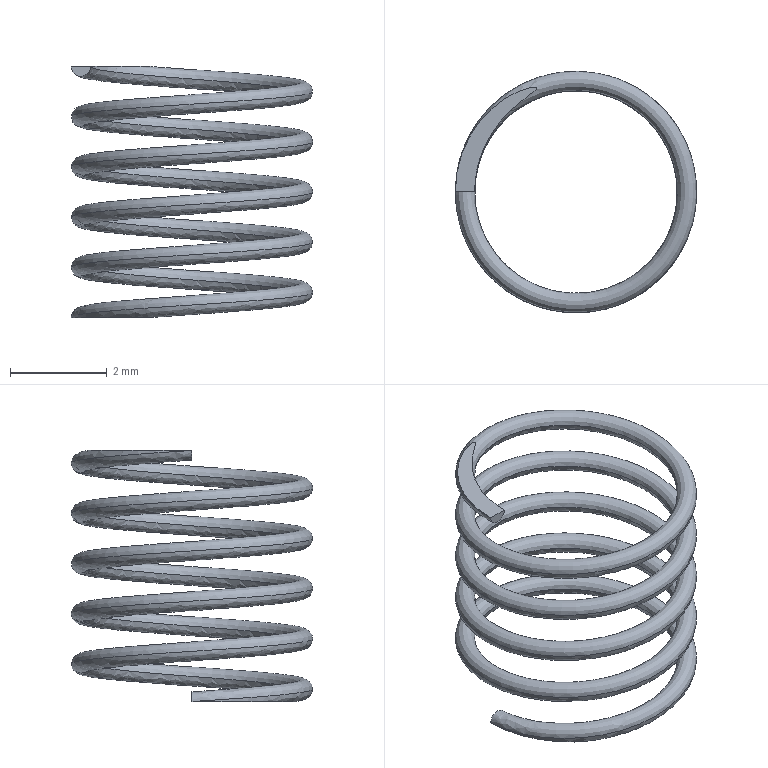Part | SolidWorks | features BaseBody 1 | 1 solid | 6 faces | box 5.001 x 5.001 x 5.2 mm | volume 8.924 mm3 | plane 4 | spline 2